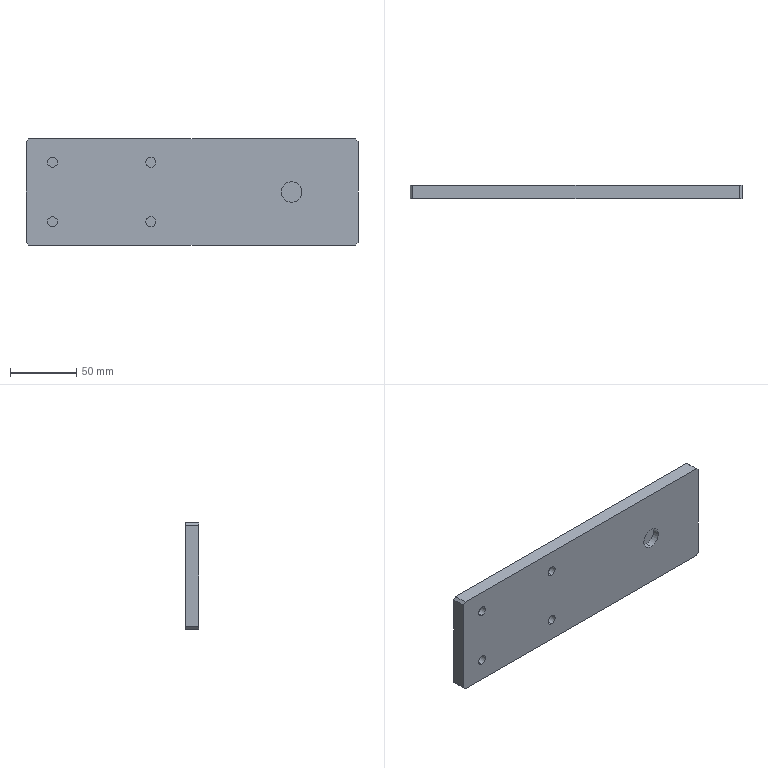Part | SolidWorks | features SplitBody 1 | 1 solid | 25 faces | box 250 x 10 x 80 mm | volume 198093 mm3 | plane 15 | cylinder 10 | commonest cylinder face diameters 7.5 x8 15.5 x2
STEP:
#1=CARTESIAN_POINT('',(500.,-58.,252.25));
#2=VERTEX_POINT('',#1);
#3=CARTESIAN_POINT('',(500.,-58.,267.75));
#4=VERTEX_POINT('',#3);
#5=CARTESIAN_POINT('',(500.,-58.,260.));
#6=DIRECTION('',(0.,1.,0.));
#7=DIRECTION('',(0.,0.,-1.));
#8=AXIS2_PLACEMENT_3D('',#5,#6,#7);
#9=CIRCLE('',#8,7.75);
#10=EDGE_CURVE('',#2,#4,#9,.T.);
#11=ORIENTED_EDGE('',*,*,#10,.T.);
#12=CARTESIAN_POINT('',(500.,-63.,267.75));
#13=VERTEX_POINT('',#12);
#14=CARTESIAN_POINT('',(500.,-58.,267.75));
#15=DIRECTION('',(0.,-1.,0.));
#16=VECTOR('',#15,1000.);
#17=LINE('',#14,#16);
#18=EDGE_CURVE('',#4,#13,#17,.T.);
#19=ORIENTED_EDGE('',*,*,#18,.T.);
#20=CARTESIAN_POINT('',(500.,-63.,252.25));
#21=VERTEX_POINT('',#20);
#22=CARTESIAN_POINT('',(500.,-63.,260.));
#23=DIRECTION('',(0.,1.,0.));
#24=DIRECTION('',(0.,0.,-1.));
#25=AXIS2_PLACEMENT_3D('',#22,#23,#24);
#26=CIRCLE('',#25,7.75);
#27=EDGE_CURVE('',#21,#13,#26,.T.);
#28=ORIENTED_EDGE('',*,*,#27,.F.);
#29=CARTESIAN_POINT('',(500.,-58.,252.25));
#30=DIRECTION('',(0.,-1.,0.));
#31=VECTOR('',#30,1000.);
#32=LINE('',#29,#31);
#33=EDGE_CURVE('',#2,#21,#32,.T.);
#34=ORIENTED_EDGE('',*,*,#33,.F.);
#35=EDGE_LOOP('',(#11,#19,#28,#34));
#36=FACE_OUTER_BOUND('',#35,.T.);
#37=CARTESIAN_POINT('',(500.,-58.,260.));
#38=DIRECTION('',(0.,-1.,0.));
#39=DIRECTION('',(0.,0.,-1.));
#40=AXIS2_PLACEMENT_3D('',#37,#38,#39);
#41=CYLINDRICAL_SURFACE('',#40,7.75);
#42=ADVANCED_FACE('',(#36),#41,.F.);
#43=CARTESIAN_POINT('',(394.,-58.,233.85));
#44=VERTEX_POINT('',#43);
#45=CARTESIAN_POINT('',(394.,-58.,241.35));
#46=VERTEX_POINT('',#45);
#47=CARTESIAN_POINT('',(394.,-58.,237.6));
#48=DIRECTION('',(0.,1.,0.));
#49=DIRECTION('',(0.,0.,-1.));
#50=AXIS2_PLACEMENT_3D('',#47,#48,#49);
#51=CIRCLE('',#50,3.75);
#52=EDGE_CURVE('',#44,#46,#51,.T.);
#53=ORIENTED_EDGE('',*,*,#52,.T.);
#54=CARTESIAN_POINT('',(394.,-63.,241.35));
#55=VERTEX_POINT('',#54);
#56=CARTESIAN_POINT('',(394.,-58.,241.35));
#57=DIRECTION('',(0.,-1.,0.));
#58=VECTOR('',#57,1000.);
#59=LINE('',#56,#58);
#60=EDGE_CURVE('',#46,#55,#59,.T.);
#61=ORIENTED_EDGE('',*,*,#60,.T.);
#62=CARTESIAN_POINT('',(394.,-63.,233.85));
#63=VERTEX_POINT('',#62);
#64=CARTESIAN_POINT('',(394.,-63.,237.6));
#65=DIRECTION('',(0.,1.,0.));
#66=DIRECTION('',(0.,0.,-1.));
#67=AXIS2_PLACEMENT_3D('',#64,#65,#66);
#68=CIRCLE('',#67,3.75);
#69=EDGE_CURVE('',#63,#55,#68,.T.);
#70=ORIENTED_EDGE('',*,*,#69,.F.);
#71=CARTESIAN_POINT('',(394.,-58.,233.85));
#72=DIRECTION('',(0.,-1.,0.));
#73=VECTOR('',#72,1000.);
#74=LINE('',#71,#73);
#75=EDGE_CURVE('',#44,#63,#74,.T.);
#76=ORIENTED_EDGE('',*,*,#75,.F.);
#77=EDGE_LOOP('',(#53,#61,#70,#76));
#78=FACE_OUTER_BOUND('',#77,.T.);
#79=CARTESIAN_POINT('',(394.,-58.,237.6));
#80=DIRECTION('',(0.,-1.,0.));
#81=DIRECTION('',(0.,0.,-1.));
#82=AXIS2_PLACEMENT_3D('',#79,#80,#81);
#83=CYLINDRICAL_SURFACE('',#82,3.75);
#84=ADVANCED_FACE('',(#78),#83,.F.);
#85=CARTESIAN_POINT('',(320.,-58.,233.85));
#86=VERTEX_POINT('',#85);
#87=CARTESIAN_POINT('',(320.,-58.,241.35));
#88=VERTEX_POINT('',#87);
#89=CARTESIAN_POINT('',(320.,-58.,237.6));
#90=DIRECTION('',(0.,1.,0.));
#91=DIRECTION('',(0.,0.,-1.));
#92=AXIS2_PLACEMENT_3D('',#89,#90,#91);
#93=CIRCLE('',#92,3.75);
#94=EDGE_CURVE('',#86,#88,#93,.T.);
#95=ORIENTED_EDGE('',*,*,#94,.T.);
#96=CARTESIAN_POINT('',(320.,-63.,241.35));
#97=VERTEX_POINT('',#96);
#98=CARTESIAN_POINT('',(320.,-58.,241.35));
#99=DIRECTION('',(0.,-1.,0.));
#100=VECTOR('',#99,1000.);
#101=LINE('',#98,#100);
#102=EDGE_CURVE('',#88,#97,#101,.T.);
#103=ORIENTED_EDGE('',*,*,#102,.T.);
#104=CARTESIAN_POINT('',(320.,-63.,233.85));
#105=VERTEX_POINT('',#104);
#106=CARTESIAN_POINT('',(320.,-63.,237.6));
#107=DIRECTION('',(0.,1.,0.));
#108=DIRECTION('',(0.,0.,-1.));
#109=AXIS2_PLACEMENT_3D('',#106,#107,#108);
#110=CIRCLE('',#109,3.75);
#111=EDGE_CURVE('',#105,#97,#110,.T.);
#112=ORIENTED_EDGE('',*,*,#111,.F.);
#113=CARTESIAN_POINT('',(320.,-58.,233.85));
#114=DIRECTION('',(0.,-1.,0.));
#115=VECTOR('',#114,1000.);
#116=LINE('',#113,#115);
#117=EDGE_CURVE('',#86,#105,#116,.T.);
#118=ORIENTED_EDGE('',*,*,#117,.F.);
#119=EDGE_LOOP('',(#95,#103,#112,#118));
#120=FACE_OUTER_BOUND('',#119,.T.);
#121=CARTESIAN_POINT('',(320.,-58.,237.6));
#122=DIRECTION('',(0.,-1.,0.));
#123=DIRECTION('',(0.,0.,-1.));
#124=AXIS2_PLACEMENT_3D('',#121,#122,#123);
#125=CYLINDRICAL_SURFACE('',#124,3.75);
#126=ADVANCED_FACE('',(#120),#125,.F.);
#127=CARTESIAN_POINT('',(320.,-58.,278.65));
#128=VERTEX_POINT('',#127);
#129=CARTESIAN_POINT('',(320.,-58.,286.15));
#130=VERTEX_POINT('',#129);
#131=CARTESIAN_POINT('',(320.,-58.,282.4));
#132=DIRECTION('',(0.,1.,0.));
#133=DIRECTION('',(0.,0.,-1.));
#134=AXIS2_PLACEMENT_3D('',#131,#132,#133);
#135=CIRCLE('',#134,3.75);
#136=EDGE_CURVE('',#128,#130,#135,.T.);
#137=ORIENTED_EDGE('',*,*,#136,.T.);
#138=CARTESIAN_POINT('',(320.,-63.,286.15));
#139=VERTEX_POINT('',#138);
#140=CARTESIAN_POINT('',(320.,-58.,286.15));
#141=DIRECTION('',(0.,-1.,0.));
#142=VECTOR('',#141,1000.);
#143=LINE('',#140,#142);
#144=EDGE_CURVE('',#130,#139,#143,.T.);
#145=ORIENTED_EDGE('',*,*,#144,.T.);
#146=CARTESIAN_POINT('',(320.,-63.,278.65));
#147=VERTEX_POINT('',#146);
#148=CARTESIAN_POINT('',(320.,-63.,282.4));
#149=DIRECTION('',(0.,1.,0.));
#150=DIRECTION('',(0.,0.,-1.));
#151=AXIS2_PLACEMENT_3D('',#148,#149,#150);
#152=CIRCLE('',#151,3.75);
#153=EDGE_CURVE('',#147,#139,#152,.T.);
#154=ORIENTED_EDGE('',*,*,#153,.F.);
#155=CARTESIAN_POINT('',(320.,-58.,278.65));
#156=DIRECTION('',(0.,-1.,0.));
#157=VECTOR('',#156,1000.);
#158=LINE('',#155,#157);
#159=EDGE_CURVE('',#128,#147,#158,.T.);
#160=ORIENTED_EDGE('',*,*,#159,.F.);
#161=EDGE_LOOP('',(#137,#145,#154,#160));
#162=FACE_OUTER_BOUND('',#161,.T.);
#163=CARTESIAN_POINT('',(320.,-58.,282.4));
#164=DIRECTION('',(0.,-1.,0.));
#165=DIRECTION('',(0.,0.,-1.));
#166=AXIS2_PLACEMENT_3D('',#163,#164,#165);
#167=CYLINDRICAL_SURFACE('',#166,3.75);
#168=ADVANCED_FACE('',(#162),#167,.F.);
#169=CARTESIAN_POINT('',(394.,-58.,278.65));
#170=VERTEX_POINT('',#169);
#171=CARTESIAN_POINT('',(394.,-58.,286.15));
#172=VERTEX_POINT('',#171);
#173=CARTESIAN_POINT('',(394.,-58.,282.4));
#174=DIRECTION('',(0.,1.,0.));
#175=DIRECTION('',(0.,0.,-1.));
#176=AXIS2_PLACEMENT_3D('',#173,#174,#175);
#177=CIRCLE('',#176,3.75);
#178=EDGE_CURVE('',#170,#172,#177,.T.);
#179=ORIENTED_EDGE('',*,*,#178,.T.);
#180=CARTESIAN_POINT('',(394.,-63.,286.15));
#181=VERTEX_POINT('',#180);
#182=CARTESIAN_POINT('',(394.,-58.,286.15));
#183=DIRECTION('',(0.,-1.,0.));
#184=VECTOR('',#183,1000.);
#185=LINE('',#182,#184);
#186=EDGE_CURVE('',#172,#181,#185,.T.);
#187=ORIENTED_EDGE('',*,*,#186,.T.);
#188=CARTESIAN_POINT('',(394.,-63.,278.65));
#189=VERTEX_POINT('',#188);
#190=CARTESIAN_POINT('',(394.,-63.,282.4));
#191=DIRECTION('',(0.,1.,0.));
#192=DIRECTION('',(0.,0.,-1.));
#193=AXIS2_PLACEMENT_3D('',#190,#191,#192);
#194=CIRCLE('',#193,3.75);
#195=EDGE_CURVE('',#189,#181,#194,.T.);
#196=ORIENTED_EDGE('',*,*,#195,.F.);
#197=CARTESIAN_POINT('',(394.,-58.,278.65));
#198=DIRECTION('',(0.,-1.,0.));
#199=VECTOR('',#198,1000.);
#200=LINE('',#197,#199);
#201=EDGE_CURVE('',#170,#189,#200,.T.);
#202=ORIENTED_EDGE('',*,*,#201,.F.);
#203=EDGE_LOOP('',(#179,#187,#196,#202));
#204=FACE_OUTER_BOUND('',#203,.T.);
#205=CARTESIAN_POINT('',(394.,-58.,282.4));
#206=DIRECTION('',(0.,-1.,0.));
#207=DIRECTION('',(0.,0.,-1.));
#208=AXIS2_PLACEMENT_3D('',#205,#206,#207);
#209=CYLINDRICAL_SURFACE('',#208,3.75);
#210=ADVANCED_FACE('',(#204),#209,.F.);
#211=CARTESIAN_POINT('',(550.,-53.,298.));
#212=VERTEX_POINT('',#211);
#213=CARTESIAN_POINT('',(550.,-53.,222.));
#214=VERTEX_POINT('',#213);
#215=CARTESIAN_POINT('',(550.,-53.,300.));
#216=DIRECTION('',(0.,0.,-1.));
#217=VECTOR('',#216,1000.);
#218=LINE('',#215,#217);
#219=EDGE_CURVE('',#212,#214,#218,.T.);
#220=ORIENTED_EDGE('',*,*,#219,.F.);
#221=CARTESIAN_POINT('',(550.,-63.,298.));
#222=VERTEX_POINT('',#221);
#223=CARTESIAN_POINT('',(550.,-63.,298.));
#224=DIRECTION('',(0.,1.,0.));
#225=VECTOR('',#224,1000.);
#226=LINE('',#223,#225);
#227=EDGE_CURVE('',#222,#212,#226,.T.);
#228=ORIENTED_EDGE('',*,*,#227,.F.);
#229=CARTESIAN_POINT('',(550.,-63.,222.));
#230=VERTEX_POINT('',#229);
#231=CARTESIAN_POINT('',(550.,-63.,300.));
#232=DIRECTION('',(0.,0.,-1.));
#233=VECTOR('',#232,1000.);
#234=LINE('',#231,#233);
#235=EDGE_CURVE('',#222,#230,#234,.T.);
#236=ORIENTED_EDGE('',*,*,#235,.T.);
#237=CARTESIAN_POINT('',(550.,-63.,222.));
#238=DIRECTION('',(0.,-1.,0.));
#239=VECTOR('',#238,1000.);
#240=LINE('',#237,#239);
#241=EDGE_CURVE('',#214,#230,#240,.T.);
#242=ORIENTED_EDGE('',*,*,#241,.F.);
#243=EDGE_LOOP('',(#220,#228,#236,#242));
#244=FACE_OUTER_BOUND('',#243,.T.);
#245=CARTESIAN_POINT('',(550.,-63.,300.));
#246=DIRECTION('',(-1.,0.,0.));
#247=DIRECTION('',(0.,1.,0.));
#248=AXIS2_PLACEMENT_3D('',#245,#246,#247);
#249=PLANE('',#248);
#250=ADVANCED_FACE('',(#244),#249,.F.);
#251=CARTESIAN_POINT('',(548.,-53.,220.));
#252=VERTEX_POINT('',#251);
#253=CARTESIAN_POINT('',(302.,-53.,220.));
#254=VERTEX_POINT('',#253);
#255=CARTESIAN_POINT('',(550.,-53.,220.));
#256=DIRECTION('',(-1.,0.,0.));
#257=VECTOR('',#256,1000.);
#258=LINE('',#255,#257);
#259=EDGE_CURVE('',#252,#254,#258,.T.);
#260=ORIENTED_EDGE('',*,*,#259,.F.);
#261=CARTESIAN_POINT('',(548.,-63.,220.));
#262=VERTEX_POINT('',#261);
#263=CARTESIAN_POINT('',(548.,-63.,220.));
#264=DIRECTION('',(0.,1.,0.));
#265=VECTOR('',#264,1000.);
#266=LINE('',#263,#265);
#267=EDGE_CURVE('',#262,#252,#266,.T.);
#268=ORIENTED_EDGE('',*,*,#267,.F.);
#269=CARTESIAN_POINT('',(302.,-63.,220.));
#270=VERTEX_POINT('',#269);
#271=CARTESIAN_POINT('',(550.,-63.,220.));
#272=DIRECTION('',(-1.,0.,0.));
#273=VECTOR('',#272,1000.);
#274=LINE('',#271,#273);
#275=EDGE_CURVE('',#262,#270,#274,.T.);
#276=ORIENTED_EDGE('',*,*,#275,.T.);
#277=CARTESIAN_POINT('',(302.,-63.,220.));
#278=DIRECTION('',(0.,-1.,0.));
#279=VECTOR('',#278,1000.);
#280=LINE('',#277,#279);
#281=EDGE_CURVE('',#254,#270,#280,.T.);
#282=ORIENTED_EDGE('',*,*,#281,.F.);
#283=EDGE_LOOP('',(#260,#268,#276,#282));
#284=FACE_OUTER_BOUND('',#283,.T.);
#285=CARTESIAN_POINT('',(550.,-63.,220.));
#286=DIRECTION('',(0.,0.,1.));
#287=DIRECTION('',(0.,-1.,0.));
#288=AXIS2_PLACEMENT_3D('',#285,#286,#287);
#289=PLANE('',#288);
#290=ADVANCED_FACE('',(#284),#289,.F.);
#291=CARTESIAN_POINT('',(300.,-63.,222.));
#292=VERTEX_POINT('',#291);
#293=CARTESIAN_POINT('',(300.,-63.,298.));
#294=VERTEX_POINT('',#293);
#295=CARTESIAN_POINT('',(300.,-63.,300.));
#296=DIRECTION('',(0.,0.,1.));
#297=VECTOR('',#296,1000.);
#298=LINE('',#295,#297);
#299=EDGE_CURVE('',#292,#294,#298,.T.);
#300=ORIENTED_EDGE('',*,*,#299,.T.);
#301=CARTESIAN_POINT('',(300.,-53.,298.));
#302=VERTEX_POINT('',#301);
#303=CARTESIAN_POINT('',(300.,-63.,298.));
#304=DIRECTION('',(0.,-1.,0.));
#305=VECTOR('',#304,1000.);
#306=LINE('',#303,#305);
#307=EDGE_CURVE('',#302,#294,#306,.T.);
#308=ORIENTED_EDGE('',*,*,#307,.F.);
#309=CARTESIAN_POINT('',(300.,-53.,222.));
#310=VERTEX_POINT('',#309);
#311=CARTESIAN_POINT('',(300.,-53.,300.));
#312=DIRECTION('',(0.,0.,1.));
#313=VECTOR('',#312,1000.);
#314=LINE('',#311,#313);
#315=EDGE_CURVE('',#310,#302,#314,.T.);
#316=ORIENTED_EDGE('',*,*,#315,.F.);
#317=CARTESIAN_POINT('',(300.,-63.,222.));
#318=DIRECTION('',(0.,1.,0.));
#319=VECTOR('',#318,1000.);
#320=LINE('',#317,#319);
#321=EDGE_CURVE('',#292,#310,#320,.T.);
#322=ORIENTED_EDGE('',*,*,#321,.F.);
#323=EDGE_LOOP('',(#300,#308,#316,#322));
#324=FACE_OUTER_BOUND('',#323,.T.);
#325=CARTESIAN_POINT('',(300.,-63.,300.));
#326=DIRECTION('',(1.,0.,0.));
#327=DIRECTION('',(0.,-1.,0.));
#328=AXIS2_PLACEMENT_3D('',#325,#326,#327);
#329=PLANE('',#328);
#330=ADVANCED_FACE('',(#324),#329,.F.);
#331=CARTESIAN_POINT('',(302.,-63.,300.));
#332=VERTEX_POINT('',#331);
#333=CARTESIAN_POINT('',(548.,-63.,300.));
#334=VERTEX_POINT('',#333);
#335=CARTESIAN_POINT('',(550.,-63.,300.));
#336=DIRECTION('',(1.,0.,0.));
#337=VECTOR('',#336,1000.);
#338=LINE('',#335,#337);
#339=EDGE_CURVE('',#332,#334,#338,.T.);
#340=ORIENTED_EDGE('',*,*,#339,.T.);
#341=CARTESIAN_POINT('',(548.,-53.,300.));
#342=VERTEX_POINT('',#341);
#343=CARTESIAN_POINT('',(548.,-63.,300.));
#344=DIRECTION('',(0.,-1.,0.));
#345=VECTOR('',#344,1000.);
#346=LINE('',#343,#345);
#347=EDGE_CURVE('',#342,#334,#346,.T.);
#348=ORIENTED_EDGE('',*,*,#347,.F.);
#349=CARTESIAN_POINT('',(302.,-53.,300.));
#350=VERTEX_POINT('',#349);
#351=CARTESIAN_POINT('',(550.,-53.,300.));
#352=DIRECTION('',(1.,0.,0.));
#353=VECTOR('',#352,1000.);
#354=LINE('',#351,#353);
#355=EDGE_CURVE('',#350,#342,#354,.T.);
#356=ORIENTED_EDGE('',*,*,#355,.F.);
#357=CARTESIAN_POINT('',(302.,-63.,300.));
#358=DIRECTION('',(0.,1.,0.));
#359=VECTOR('',#358,1000.);
#360=LINE('',#357,#359);
#361=EDGE_CURVE('',#332,#350,#360,.T.);
#362=ORIENTED_EDGE('',*,*,#361,.F.);
#363=EDGE_LOOP('',(#340,#348,#356,#362));
#364=FACE_OUTER_BOUND('',#363,.T.);
#365=CARTESIAN_POINT('',(550.,-63.,300.));
#366=DIRECTION('',(0.,0.,-1.));
#367=DIRECTION('',(0.,1.,0.));
#368=AXIS2_PLACEMENT_3D('',#365,#366,#367);
#369=PLANE('',#368);
#370=ADVANCED_FACE('',(#364),#369,.F.);
#371=ORIENTED_EDGE('',*,*,#27,.T.);
#372=CARTESIAN_POINT('',(500.,-63.,260.));
#373=DIRECTION('',(0.,1.,0.));
#374=DIRECTION('',(0.,0.,-1.));
#375=AXIS2_PLACEMENT_3D('',#372,#373,#374);
#376=CIRCLE('',#375,7.75);
#377=EDGE_CURVE('',#13,#21,#376,.T.);
#378=ORIENTED_EDGE('',*,*,#377,.T.);
#379=EDGE_LOOP('',(#371,#378));
#380=FACE_BOUND('',#379,.T.);
#381=ORIENTED_EDGE('',*,*,#69,.T.);
#382=CARTESIAN_POINT('',(394.,-63.,237.6));
#383=DIRECTION('',(0.,1.,0.));
#384=DIRECTION('',(0.,0.,-1.));
#385=AXIS2_PLACEMENT_3D('',#382,#383,#384);
#386=CIRCLE('',#385,3.75);
#387=EDGE_CURVE('',#55,#63,#386,.T.);
#388=ORIENTED_EDGE('',*,*,#387,.T.);
#389=EDGE_LOOP('',(#381,#388));
#390=FACE_BOUND('',#389,.T.);
#391=ORIENTED_EDGE('',*,*,#111,.T.);
#392=CARTESIAN_POINT('',(320.,-63.,237.6));
#393=DIRECTION('',(0.,1.,0.));
#394=DIRECTION('',(0.,0.,-1.));
#395=AXIS2_PLACEMENT_3D('',#392,#393,#394);
#396=CIRCLE('',#395,3.75);
#397=EDGE_CURVE('',#97,#105,#396,.T.);
#398=ORIENTED_EDGE('',*,*,#397,.T.);
#399=EDGE_LOOP('',(#391,#398));
#400=FACE_BOUND('',#399,.T.);
#401=ORIENTED_EDGE('',*,*,#153,.T.);
#402=CARTESIAN_POINT('',(320.,-63.,282.4));
#403=DIRECTION('',(0.,1.,0.));
#404=DIRECTION('',(0.,0.,-1.));
#405=AXIS2_PLACEMENT_3D('',#402,#403,#404);
#406=CIRCLE('',#405,3.75);
#407=EDGE_CURVE('',#139,#147,#406,.T.);
#408=ORIENTED_EDGE('',*,*,#407,.T.);
#409=EDGE_LOOP('',(#401,#408));
#410=FACE_BOUND('',#409,.T.);
#411=ORIENTED_EDGE('',*,*,#195,.T.);
#412=CARTESIAN_POINT('',(394.,-63.,282.4));
#413=DIRECTION('',(0.,1.,0.));
#414=DIRECTION('',(0.,0.,-1.));
#415=AXIS2_PLACEMENT_3D('',#412,#413,#414);
#416=CIRCLE('',#415,3.75);
#417=EDGE_CURVE('',#181,#189,#416,.T.);
#418=ORIENTED_EDGE('',*,*,#417,.T.);
#419=EDGE_LOOP('',(#411,#418));
#420=FACE_BOUND('',#419,.T.);
#421=ORIENTED_EDGE('',*,*,#275,.F.);
#422=CARTESIAN_POINT('',(164.,-63.,-164.));
#423=DIRECTION('',(-0.7071,0.,-0.7071));
#424=VECTOR('',#423,1000.);
#425=LINE('',#422,#424);
#426=EDGE_CURVE('',#230,#262,#425,.T.);
#427=ORIENTED_EDGE('',*,*,#426,.F.);
#428=ORIENTED_EDGE('',*,*,#235,.F.);
#429=CARTESIAN_POINT('',(424.,-63.,424.));
#430=DIRECTION('',(0.7071,0.,-0.7071));
#431=VECTOR('',#430,1000.);
#432=LINE('',#429,#431);
#433=EDGE_CURVE('',#334,#222,#432,.T.);
#434=ORIENTED_EDGE('',*,*,#433,.F.);
#435=ORIENTED_EDGE('',*,*,#339,.F.);
#436=CARTESIAN_POINT('',(1.,-63.,-1.));
#437=DIRECTION('',(0.7071,0.,0.7071));
#438=VECTOR('',#437,1000.);
#439=LINE('',#436,#438);
#440=EDGE_CURVE('',#294,#332,#439,.T.);
#441=ORIENTED_EDGE('',*,*,#440,.F.);
#442=ORIENTED_EDGE('',*,*,#299,.F.);
#443=CARTESIAN_POINT('',(261.,-63.,261.));
#444=DIRECTION('',(-0.7071,0.,0.7071));
#445=VECTOR('',#444,1000.);
#446=LINE('',#443,#445);
#447=EDGE_CURVE('',#270,#292,#446,.T.);
#448=ORIENTED_EDGE('',*,*,#447,.F.);
#449=EDGE_LOOP('',(#421,#427,#428,#434,#435,#441,#442,#448));
#450=FACE_OUTER_BOUND('',#449,.T.);
#451=CARTESIAN_POINT('',(0.,-63.,0.));
#452=DIRECTION('',(0.,-1.,0.));
#453=DIRECTION('',(0.,0.,-1.));
#454=AXIS2_PLACEMENT_3D('',#451,#452,#453);
#455=PLANE('',#454);
#456=ADVANCED_FACE('',(#380,#390,#400,#410,#420,#450),#455,.T.);
#457=ORIENTED_EDGE('',*,*,#315,.T.);
#458=CARTESIAN_POINT('',(302.,-53.,300.));
#459=DIRECTION('',(-0.7071,0.,-0.7071));
#460=VECTOR('',#459,1000.);
#461=LINE('',#458,#460);
#462=EDGE_CURVE('',#350,#302,#461,.T.);
#463=ORIENTED_EDGE('',*,*,#462,.F.);
#464=ORIENTED_EDGE('',*,*,#355,.T.);
#465=CARTESIAN_POINT('',(550.,-53.,298.));
#466=DIRECTION('',(-0.7071,0.,0.7071));
#467=VECTOR('',#466,1000.);
#468=LINE('',#465,#467);
#469=EDGE_CURVE('',#212,#342,#468,.T.);
#470=ORIENTED_EDGE('',*,*,#469,.F.);
#471=ORIENTED_EDGE('',*,*,#219,.T.);
#472=CARTESIAN_POINT('',(548.,-53.,220.));
#473=DIRECTION('',(0.7071,0.,0.7071));
#474=VECTOR('',#473,1000.);
#475=LINE('',#472,#474);
#476=EDGE_CURVE('',#252,#214,#475,.T.);
#477=ORIENTED_EDGE('',*,*,#476,.F.);
#478=ORIENTED_EDGE('',*,*,#259,.T.);
#479=CARTESIAN_POINT('',(300.,-53.,222.));
#480=DIRECTION('',(0.7071,0.,-0.7071));
#481=VECTOR('',#480,1000.);
#482=LINE('',#479,#481);
#483=EDGE_CURVE('',#310,#254,#482,.T.);
#484=ORIENTED_EDGE('',*,*,#483,.F.);
#485=EDGE_LOOP('',(#457,#463,#464,#470,#471,#477,#478,#484));
#486=FACE_OUTER_BOUND('',#485,.T.);
#487=CARTESIAN_POINT('',(0.,-53.,0.));
#488=DIRECTION('',(0.,-1.,0.));
#489=DIRECTION('',(0.,0.,-1.));
#490=AXIS2_PLACEMENT_3D('',#487,#488,#489);
#491=PLANE('',#490);
#492=ADVANCED_FACE('',(#486),#491,.F.);
#493=ORIENTED_EDGE('',*,*,#186,.F.);
#494=CARTESIAN_POINT('',(394.,-58.,282.4));
#495=DIRECTION('',(0.,1.,0.));
#496=DIRECTION('',(0.,0.,-1.));
#497=AXIS2_PLACEMENT_3D('',#494,#495,#496);
#498=CIRCLE('',#497,3.75);
#499=EDGE_CURVE('',#172,#170,#498,.T.);
#500=ORIENTED_EDGE('',*,*,#499,.T.);
#501=ORIENTED_EDGE('',*,*,#201,.T.);
#502=ORIENTED_EDGE('',*,*,#417,.F.);
#503=EDGE_LOOP('',(#493,#500,#501,#502));
#504=FACE_OUTER_BOUND('',#503,.T.);
#505=CARTESIAN_POINT('',(394.,-58.,282.4));
#506=DIRECTION('',(0.,-1.,0.));
#507=DIRECTION('',(0.,0.,-1.));
#508=AXIS2_PLACEMENT_3D('',#505,#506,#507);
#509=CYLINDRICAL_SURFACE('',#508,3.75);
#510=ADVANCED_FACE('',(#504),#509,.F.);
#511=ORIENTED_EDGE('',*,*,#178,.F.);
#512=ORIENTED_EDGE('',*,*,#499,.F.);
#513=EDGE_LOOP('',(#511,#512));
#514=FACE_OUTER_BOUND('',#513,.T.);
#515=CARTESIAN_POINT('',(394.,-58.,282.4));
#516=DIRECTION('',(0.,-1.,0.));
#517=DIRECTION('',(0.,0.,-1.));
#518=AXIS2_PLACEMENT_3D('',#515,#516,#517);
#519=PLANE('',#518);
#520=ADVANCED_FACE('',(#514),#519,.T.);
#521=ORIENTED_EDGE('',*,*,#144,.F.);
#522=CARTESIAN_POINT('',(320.,-58.,282.4));
#523=DIRECTION('',(0.,1.,0.));
#524=DIRECTION('',(0.,0.,-1.));
#525=AXIS2_PLACEMENT_3D('',#522,#523,#524);
#526=CIRCLE('',#525,3.75);
#527=EDGE_CURVE('',#130,#128,#526,.T.);
#528=ORIENTED_EDGE('',*,*,#527,.T.);
#529=ORIENTED_EDGE('',*,*,#159,.T.);
#530=ORIENTED_EDGE('',*,*,#407,.F.);
#531=EDGE_LOOP('',(#521,#528,#529,#530));
#532=FACE_OUTER_BOUND('',#531,.T.);
#533=CARTESIAN_POINT('',(320.,-58.,282.4));
#534=DIRECTION('',(0.,-1.,0.));
#535=DIRECTION('',(0.,0.,-1.));
#536=AXIS2_PLACEMENT_3D('',#533,#534,#535);
#537=CYLINDRICAL_SURFACE('',#536,3.75);
#538=ADVANCED_FACE('',(#532),#537,.F.);
#539=ORIENTED_EDGE('',*,*,#136,.F.);
#540=ORIENTED_EDGE('',*,*,#527,.F.);
#541=EDGE_LOOP('',(#539,#540));
#542=FACE_OUTER_BOUND('',#541,.T.);
#543=CARTESIAN_POINT('',(320.,-58.,282.4));
#544=DIRECTION('',(0.,-1.,0.));
#545=DIRECTION('',(0.,0.,-1.));
#546=AXIS2_PLACEMENT_3D('',#543,#544,#545);
#547=PLANE('',#546);
#548=ADVANCED_FACE('',(#542),#547,.T.);
#549=ORIENTED_EDGE('',*,*,#102,.F.);
#550=CARTESIAN_POINT('',(320.,-58.,237.6));
#551=DIRECTION('',(0.,1.,0.));
#552=DIRECTION('',(0.,0.,-1.));
#553=AXIS2_PLACEMENT_3D('',#550,#551,#552);
#554=CIRCLE('',#553,3.75);
#555=EDGE_CURVE('',#88,#86,#554,.T.);
#556=ORIENTED_EDGE('',*,*,#555,.T.);
#557=ORIENTED_EDGE('',*,*,#117,.T.);
#558=ORIENTED_EDGE('',*,*,#397,.F.);
#559=EDGE_LOOP('',(#549,#556,#557,#558));
#560=FACE_OUTER_BOUND('',#559,.T.);
#561=CARTESIAN_POINT('',(320.,-58.,237.6));
#562=DIRECTION('',(0.,-1.,0.));
#563=DIRECTION('',(0.,0.,-1.));
#564=AXIS2_PLACEMENT_3D('',#561,#562,#563);
#565=CYLINDRICAL_SURFACE('',#564,3.75);
#566=ADVANCED_FACE('',(#560),#565,.F.);
#567=ORIENTED_EDGE('',*,*,#94,.F.);
#568=ORIENTED_EDGE('',*,*,#555,.F.);
#569=EDGE_LOOP('',(#567,#568));
#570=FACE_OUTER_BOUND('',#569,.T.);
#571=CARTESIAN_POINT('',(320.,-58.,237.6));
#572=DIRECTION('',(0.,-1.,0.));
#573=DIRECTION('',(0.,0.,-1.));
#574=AXIS2_PLACEMENT_3D('',#571,#572,#573);
#575=PLANE('',#574);
#576=ADVANCED_FACE('',(#570),#575,.T.);
#577=ORIENTED_EDGE('',*,*,#60,.F.);
#578=CARTESIAN_POINT('',(394.,-58.,237.6));
#579=DIRECTION('',(0.,1.,0.));
#580=DIRECTION('',(0.,0.,-1.));
#581=AXIS2_PLACEMENT_3D('',#578,#579,#580);
#582=CIRCLE('',#581,3.75);
#583=EDGE_CURVE('',#46,#44,#582,.T.);
#584=ORIENTED_EDGE('',*,*,#583,.T.);
#585=ORIENTED_EDGE('',*,*,#75,.T.);
#586=ORIENTED_EDGE('',*,*,#387,.F.);
#587=EDGE_LOOP('',(#577,#584,#585,#586));
#588=FACE_OUTER_BOUND('',#587,.T.);
#589=CARTESIAN_POINT('',(394.,-58.,237.6));
#590=DIRECTION('',(0.,-1.,0.));
#591=DIRECTION('',(0.,0.,-1.));
#592=AXIS2_PLACEMENT_3D('',#589,#590,#591);
#593=CYLINDRICAL_SURFACE('',#592,3.75);
#594=ADVANCED_FACE('',(#588),#593,.F.);
#595=ORIENTED_EDGE('',*,*,#52,.F.);
#596=ORIENTED_EDGE('',*,*,#583,.F.);
#597=EDGE_LOOP('',(#595,#596));
#598=FACE_OUTER_BOUND('',#597,.T.);
#599=CARTESIAN_POINT('',(394.,-58.,237.6));
#600=DIRECTION('',(0.,-1.,0.));
#601=DIRECTION('',(0.,0.,-1.));
#602=AXIS2_PLACEMENT_3D('',#599,#600,#601);
#603=PLANE('',#602);
#604=ADVANCED_FACE('',(#598),#603,.T.);
#605=ORIENTED_EDGE('',*,*,#447,.T.);
#606=ORIENTED_EDGE('',*,*,#321,.T.);
#607=ORIENTED_EDGE('',*,*,#483,.T.);
#608=ORIENTED_EDGE('',*,*,#281,.T.);
#609=EDGE_LOOP('',(#605,#606,#607,#608));
#610=FACE_OUTER_BOUND('',#609,.T.);
#611=CARTESIAN_POINT('',(300.,-63.,222.));
#612=DIRECTION('',(0.7071,0.,0.7071));
#613=DIRECTION('',(0.,1.,0.));
#614=AXIS2_PLACEMENT_3D('',#611,#612,#613);
#615=PLANE('',#614);
#616=ADVANCED_FACE('',(#610),#615,.F.);
#617=ORIENTED_EDGE('',*,*,#440,.T.);
#618=ORIENTED_EDGE('',*,*,#361,.T.);
#619=ORIENTED_EDGE('',*,*,#462,.T.);
#620=ORIENTED_EDGE('',*,*,#307,.T.);
#621=EDGE_LOOP('',(#617,#618,#619,#620));
#622=FACE_OUTER_BOUND('',#621,.T.);
#623=CARTESIAN_POINT('',(302.,-63.,300.));
#624=DIRECTION('',(0.7071,0.,-0.7071));
#625=DIRECTION('',(0.,1.,0.));
#626=AXIS2_PLACEMENT_3D('',#623,#624,#625);
#627=PLANE('',#626);
#628=ADVANCED_FACE('',(#622),#627,.F.);
#629=ORIENTED_EDGE('',*,*,#426,.T.);
#630=ORIENTED_EDGE('',*,*,#267,.T.);
#631=ORIENTED_EDGE('',*,*,#476,.T.);
#632=ORIENTED_EDGE('',*,*,#241,.T.);
#633=EDGE_LOOP('',(#629,#630,#631,#632));
#634=FACE_OUTER_BOUND('',#633,.T.);
#635=CARTESIAN_POINT('',(548.,-63.,220.));
#636=DIRECTION('',(-0.7071,0.,0.7071));
#637=DIRECTION('',(0.,1.,0.));
#638=AXIS2_PLACEMENT_3D('',#635,#636,#637);
#639=PLANE('',#638);
#640=ADVANCED_FACE('',(#634),#639,.F.);
#641=ORIENTED_EDGE('',*,*,#433,.T.);
#642=ORIENTED_EDGE('',*,*,#227,.T.);
#643=ORIENTED_EDGE('',*,*,#469,.T.);
#644=ORIENTED_EDGE('',*,*,#347,.T.);
#645=EDGE_LOOP('',(#641,#642,#643,#644));
#646=FACE_OUTER_BOUND('',#645,.T.);
#647=CARTESIAN_POINT('',(550.,-63.,298.));
#648=DIRECTION('',(-0.7071,0.,-0.7071));
#649=DIRECTION('',(0.,1.,0.));
#650=AXIS2_PLACEMENT_3D('',#647,#648,#649);
#651=PLANE('',#650);
#652=ADVANCED_FACE('',(#646),#651,.F.);
#653=ORIENTED_EDGE('',*,*,#18,.F.);
#654=CARTESIAN_POINT('',(500.,-58.,260.));
#655=DIRECTION('',(0.,1.,0.));
#656=DIRECTION('',(0.,0.,-1.));
#657=AXIS2_PLACEMENT_3D('',#654,#655,#656);
#658=CIRCLE('',#657,7.75);
#659=EDGE_CURVE('',#4,#2,#658,.T.);
#660=ORIENTED_EDGE('',*,*,#659,.T.);
#661=ORIENTED_EDGE('',*,*,#33,.T.);
#662=ORIENTED_EDGE('',*,*,#377,.F.);
#663=EDGE_LOOP('',(#653,#660,#661,#662));
#664=FACE_OUTER_BOUND('',#663,.T.);
#665=CARTESIAN_POINT('',(500.,-58.,260.));
#666=DIRECTION('',(0.,-1.,0.));
#667=DIRECTION('',(0.,0.,-1.));
#668=AXIS2_PLACEMENT_3D('',#665,#666,#667);
#669=CYLINDRICAL_SURFACE('',#668,7.75);
#670=ADVANCED_FACE('',(#664),#669,.F.);
#671=ORIENTED_EDGE('',*,*,#10,.F.);
#672=ORIENTED_EDGE('',*,*,#659,.F.);
#673=EDGE_LOOP('',(#671,#672));
#674=FACE_OUTER_BOUND('',#673,.T.);
#675=CARTESIAN_POINT('',(500.,-58.,260.));
#676=DIRECTION('',(0.,-1.,0.));
#677=DIRECTION('',(0.,0.,-1.));
#678=AXIS2_PLACEMENT_3D('',#675,#676,#677);
#679=PLANE('',#678);
#680=ADVANCED_FACE('',(#674),#679,.T.);
#681=CLOSED_SHELL('',(#42,#84,#126,#168,#210,#250,#290,#330,#370,#456,#492,#510,#520,#538,#548,#566,#576,#594,#604,#616,#628,#640,#652,#670,#680));
#682=MANIFOLD_SOLID_BREP('',#681);
#683=CARTESIAN_POINT('',(0.,0.,0.));
#684=DIRECTION('',(0.,0.,1.));
#685=DIRECTION('',(1.,0.,0.));
#686=AXIS2_PLACEMENT_3D('',#683,#684,#685);
#687=(LENGTH_UNIT()NAMED_UNIT(*)SI_UNIT(.MILLI.,.METRE.));
#688=UNCERTAINTY_MEASURE_WITH_UNIT(LENGTH_MEASURE(0.00001),#687,'','');
#689=(NAMED_UNIT(*)PLANE_ANGLE_UNIT()SI_UNIT($,.RADIAN.));
#690=(NAMED_UNIT(*)SI_UNIT($,.STERADIAN.)SOLID_ANGLE_UNIT());
#691=(GEOMETRIC_REPRESENTATION_CONTEXT(3)GLOBAL_UNCERTAINTY_ASSIGNED_CONTEXT((#688))GLOBAL_UNIT_ASSIGNED_CONTEXT((#687,#689,#690))REPRESENTATION_CONTEXT('',''));
#692=ADVANCED_BREP_SHAPE_REPRESENTATION('',(#682,#686),#691);